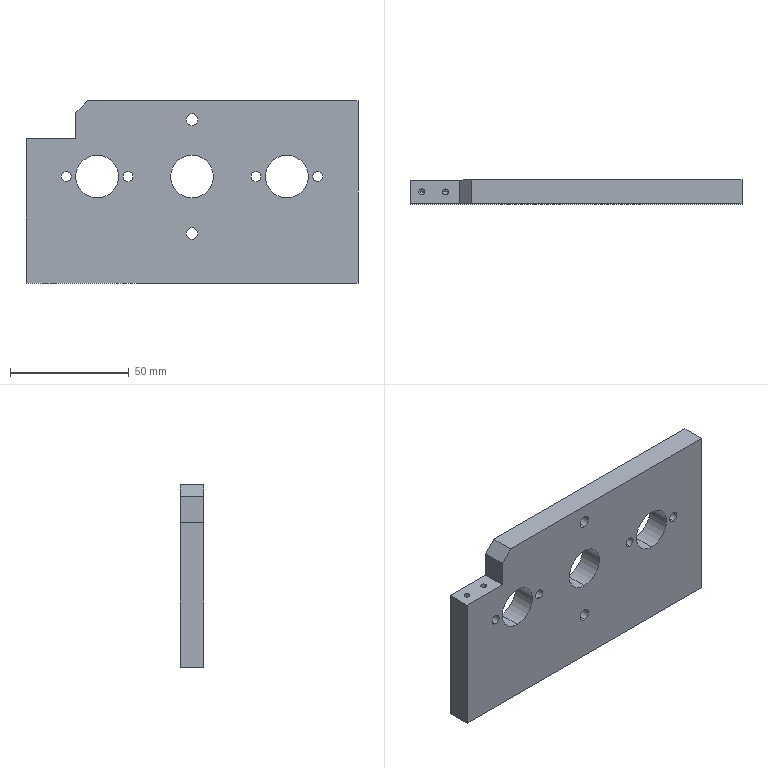Part | STEP file | 0232_202_Plate | 1 solid | 51 faces | box 140 x 10 x 77 mm | volume 94013 mm3 | cylinder 30 | cone 12 | plane 9 | commonest cylinder face diameters 5 x12 4.2 x8 18 x6 2.5 x4